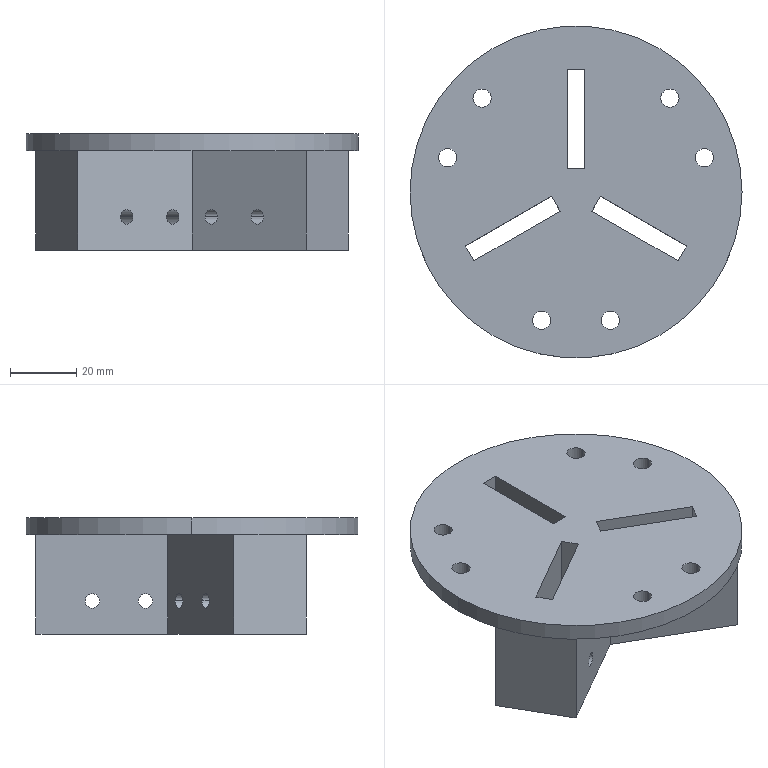Part | SolidWorks | features ICE 6, CirPattern 2, Extrusion 1 | 1 solid | 80 faces | box 100 x 100 x 35 mm | volume 118431 mm3 | cylinder 50 | plane 30 | commonest cylinder face diameters 4.4 x24 5.5 x12 12 x12 100 x2